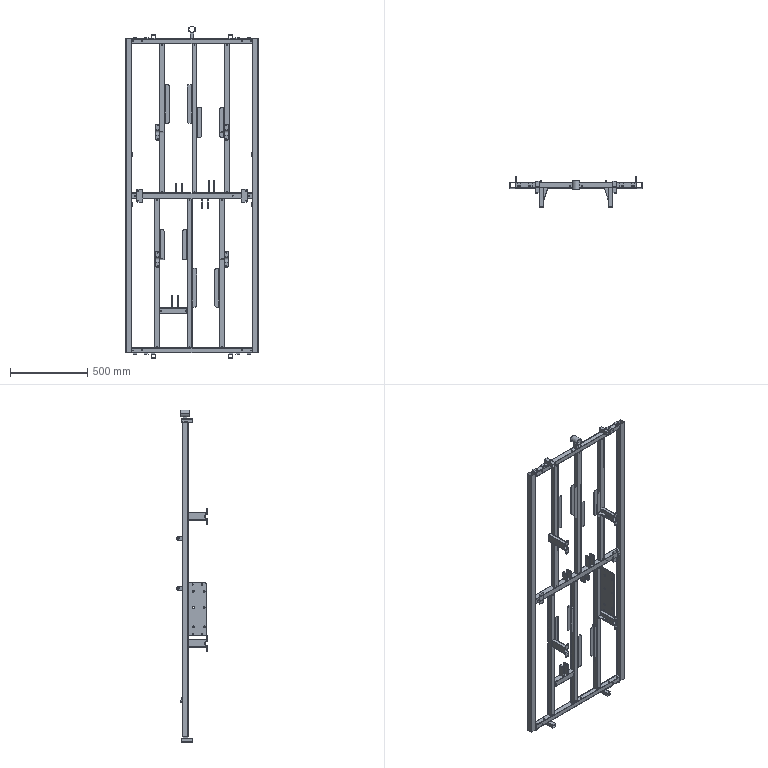Part | NX | features BREP 23 | 65 solids | 1062 faces | box 856.234 x 200.406 x 2148 mm | volume 4023122 mm3 | plane 598 | cylinder 460 | spline 4 | commonest cylinder face diameters 3.175 x100 8.128 x56 10.16 x32 19.05 x32 4.763 x24 6.604 x16